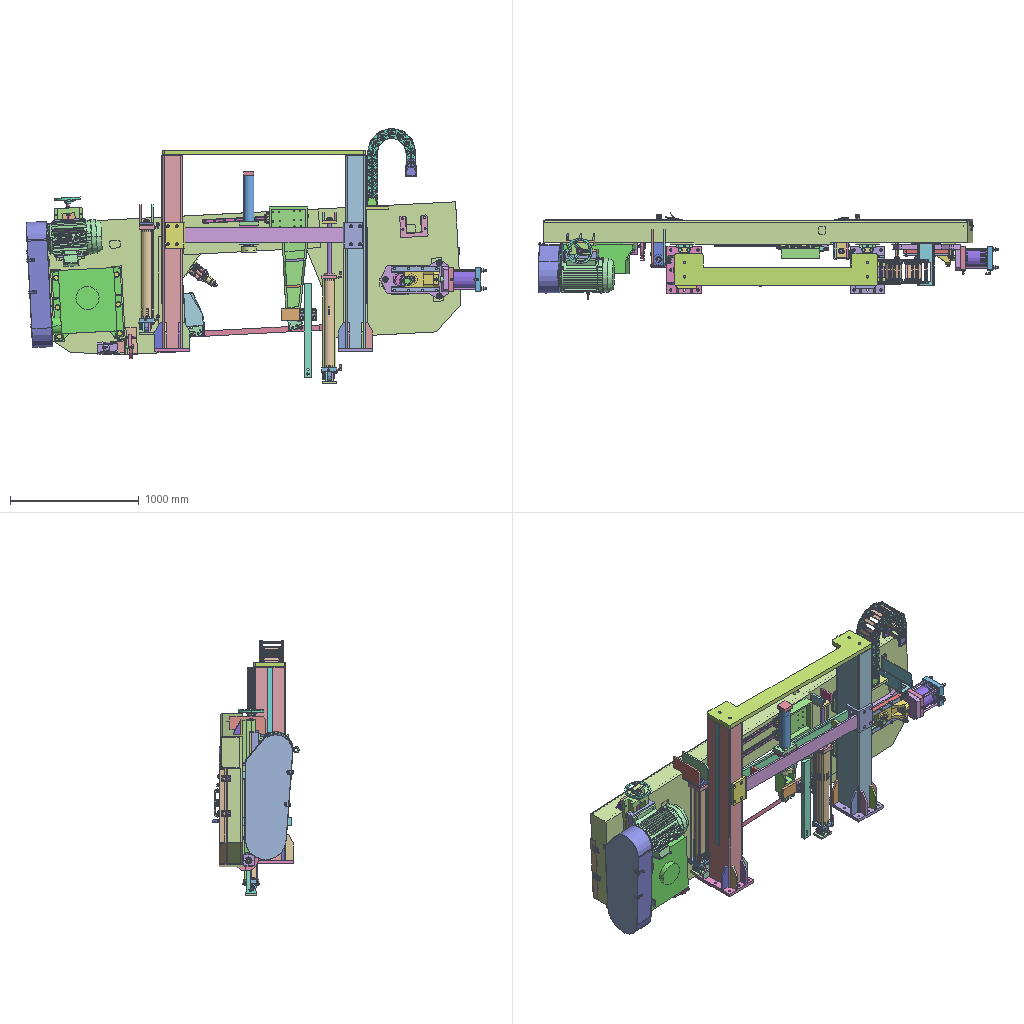Assembly | SolidWorks | 178 different items | 453 placed | box 3568 x 670 x 1981 mm
Parts list (item | name | quantity | parent item | size | volume | features):
1 | (subassembly) | x6 | in 21 | 75 x 44 x 44 mm | 50797 mm3 | -
2 | (subassembly) | x1 | - | - | 3103093 mm3 | features ReferencePattern 10, CompositeCurve 2, LocalChainPattern 1
3 | (subassembly) | x1 | in 2 | 145.118 x 185 x 82 mm | 205797 mm3 | features MirrorCompFeat 1, ReferencePattern 1
4 | (subassembly) | x11 | in 2 | 152 x 185 x 74 mm | 243841 mm3 | -
5 | (subassembly) | x1 | in 2 | 142.639 x 185 x 82 mm | 215082 mm3 | features MirrorCompFeat 1, ReferencePattern 1
6 | (subassembly) | x1 | - | 1530 x 622 x 137.5 mm | 11760878 mm3 | -
7 | (subassembly) | x1 | in 6 | 150 x 120 x 674.743 mm | 3033586 mm3 | -
8 | (subassembly) | x1 | - | - | 208271945 mm3 | features CompositeCurve 6
9 | (subassembly) | x1 | - | 159.892 x 293.5 x 1004 mm | 4407158 mm3 | features MirrorCompFeat 2, ReferencePattern 2
10 | (subassembly) | x1 | in 12 | 113.1 x 154 x 66 mm | 527835 mm3 | features ReferencePattern 4, MirrorCompFeat 1
11 | (subassembly) | x1 | in 9 | 159.892 x 127 x 873 mm | 2737891 mm3 | features ReferencePattern 9, LocalCirPattern 1
12 | (subassembly) | x1 | - | 1034 x 251 x 1320 mm | 13536578 mm3 | features CompositeCurve 1
13 | (subassembly) | x1 | - | 159.892 x 128.5 x 1129 mm | 3522058 mm3 | features MirrorCompFeat 2, ReferencePattern 2
14 | (subassembly) | x1 | in 12 | 113.1 x 154 x 66 mm | 527835 mm3 | features ReferencePattern 4, MirrorCompFeat 1
15 | (subassembly) | x1 | in 12 | 275 x 90 x 76.5 mm | 961874 mm3 | features ReferencePattern 13, LocalLPattern 1, MirrorCompFeat 1
16 | (subassembly) | x1 | - | 818.008 x 265.16 x 304.212 mm | 12071604 mm3 | features ReferencePattern 8, LocalLPattern 1, MirrorCompFeat 1
17 | (subassembly) | x6 | in 8 | 95.983 x 31.176 x 12 mm | 3413 mm3 | -
18 | (subassembly) | x1 | in 8 | 558.147 x 472.8 x 532.819 mm | 28170554 mm3 | features ReferencePattern 2, LocalLPattern 1, MirrorCompFeat 1
19 | (subassembly) | x1 | - | 1815 x 380 x 1565 mm | 40801474 mm3 | -
20 | (subassembly) | x1 | in 8 | 141.618 x 147.365 x 259.286 mm | 1445767 mm3 | -
21 | (subassembly) | x1 | in 8 | 690 x 549 x 426.5 mm | 59127815 mm3 | features ReferencePattern 3, MirrorCompFeat 1
22 | (subassembly) | x1 | in 13 | 159.892 x 127 x 1033 mm | 2737892 mm3 | features ReferencePattern 9, LocalCirPattern 1
23 | (subassembly) | x1 | in 8 | 280.7 x 140.048 x 94.951 mm | 1394120 mm3 | -
24 | (subassembly) | x1 | in 16 | 180 x 218.16 x 499.969 mm | 4201061 mm3 | features ReferencePattern 6, LocalCirPattern 1
25 | (subassembly) | x2 | in 8 | 90 x 42 x 820 mm | 939194 mm3 | features LocalLPattern 1, ReferencePattern 1
26 | (subassembly) | x1 | in 19 | 120 x 60 x 1330 mm | 3294670 mm3 | features LocalLPattern 1, ReferencePattern 1
27 | (subassembly) | x1 | in 19 | 120 x 60 x 1330 mm | 3294670 mm3 | features LocalLPattern 1, ReferencePattern 1
28 | (subassembly) | x8 | in 16 | 20 x 20 x 41.4 mm | 4793 mm3 | -
29 | (subassembly) | x4 | in 18 | 37.5 x 24 x 24 mm | 6610 mm3 | -
30 | (subassembly) | x4 | in 24 | 30 x 30 x 21.9 mm | 7598 mm3 | -
31 | - | x6 | in 17 | 56.004 x 15.265 x 22.5 mm | 1517 mm3 | features BaseBody 1
32 | - | x1 | in 24 | 180 x 180 x 56 mm | 1310949 mm3 | features ICE 4, RevCut 2, Extrusion 1, HoleWzd 1
33 | - | x1 | in 24 | 180 x 180 x 56 mm | 1375420 mm3 | features ICE 4, Extrusion 1, HoleWzd 1, RevCut 1
34 | - | x1 | in 24 | 40 x 150 x 150 mm | 516029 mm3 | features Chamfer 1, Revolution 1
35 | - | x1 | in 16 | 265 x 175 x 150 mm | 1974640 mm3 | features ICE 8, Chamfer 2, 3DProfileFeature 1, Extrusion 1, HoleWzd 1, RevCut 1
36 | - | x1 | in 16 | 526.008 x 205 x 304.212 mm | 5277088 mm3 | features ICE 7, HoleWzd 3, 3DProfileFeature 1, Extrusion 1, Fillet 1, WeldmentFeature 1
37 | - | x1 | in 18 | 45 x 200 x 200 mm | 211717 mm3 | features ICE 2, CirPattern 1, Revolution 1, Sweep 1
38 | - | x1 | - | 212 x 330 x 165 mm | 621985 mm3 | features ICE 3, Fillet 2, EdgeFlange 1, FlatPattern 1, HoleWzd 1, SMBaseFlange 1, SheetMetal 1
39 | - | x2 | in 8 | 138.654 x 37 x 27 mm | 43785 mm3 | features ICE 6, Extrusion 1
40 | - | x1 | in 8 | 34 x 10 x 100 mm | 16950 mm3 | features MBimport 1
41 | - | x1 | in 7 | 150 x 100 x 40 mm | 435431 mm3 | features ICE 3, Extrusion 1
42 | - | x2 | in 10, 14 | 6 x 6 x 26 mm | 614.212 mm3 | features Chamfer 2, Cut 2, Extrusion 1, RevCut 1, Revolution 1
43 | - | x1 | in 7 | 80 x 80 x 40 mm | 223172 mm3 | features Extrusion 1, ICE 1
44 | - | x1 | in 7 | 70 x 70 x 40 mm | 58905 mm3 | features Extrusion 1
45 | - | x1 | in 7 | 572 x 60 x 60 mm | 1573135 mm3 | features Revolution 1
46 | - | x1 | in 7 | 80 x 80 x 360 mm | 424115 mm3 | features Extrusion 1
47 | - | x1 | in 23 | 242.5 x 94.951 x 94.951 mm | 1199171 mm3 | features MBimport 1
48 | - | x1 | in 23 | 25 x 25 x 60 mm | 21851 mm3 | features Extrusion 1, ICE 1, RevCut 1
49 | - | x2 | in 18 | 50 x 290 x 20 mm | 282397 mm3 | features Extrusion 1, HoleWzd 1
50 | - | x1 | in 18 | 240 x 51 x 290 mm | 2244437 mm3 | features HoleWzd 2, Extrusion 1, ICE 1
51 | - | x1 | in 18 | 215 x 95 x 400 mm | 2889369 mm3 | features ICE 4, Extrusion 1, HoleWzd 1
52 | - | x1 | in 18 | 350.5 x 38 x 38 mm | 174413 mm3 | features Chamfer 1, ICE 1, Revolution 1
53 | - | x6 | in 10, 14 | 9 x 30 x 30 mm | 4367 mm3 | features Revolution 3, CirPattern 1, RefAxis 1
54 | - | x1 | in 18 | 50 x 60 x 73 mm | 158033 mm3 | features Chamfer 1, Extrusion 1, HoleWzd 1, ICE 1
55 | - | x2 | in 8 | 238 x 839.181 x 17 mm | 391508 mm3 | features Sweep 1
56 | - | x1 | in 8 | 163 x 973.632 x 386.5 mm | 1244808 mm3 | features ICE 7, Extrusion 1, HoleWzd 1, WeldBeadFeat 1, WeldmentFeature 1
57 | - | x2 | in 8 | 60 x 380 x 10 mm | 228000 mm3 | features Extrusion 1
58 | - | x1 | in 8 | 386.5 x 973.632 x 16 mm | 607839 mm3 | features ICE 3, Extrusion 1, WeldmentFeature 1
59 | - | x1 | - | 1570 x 250 x 35 mm | 9261323 mm3 | features SavedExtBody 1
60 | - | x1 | in 19 | 1570 x 250 x 35 mm | 9261323 mm3 | features Cut 2, Extrusion 1, Fillet 1
61 | - | x2 | in 10, 14 | 11 x 16 x 39 mm | 6238 mm3 | features ICE 2, Extrusion 1
62 | - | x2 | in 9, 13 | 47 x 22 x 47 mm | 19543 mm3 | features Revolution 2
63 | - | x3 | in 16 | 128 x 36 x 41.569 mm | 67364 mm3 | features ICE 2, Extrusion 1, RevCut 1, Revolution 1
64 | - | x8 | in 15 | 11 x 35 x 35 mm | 6620 mm3 | features Revolution 3, CirPattern 1, RefAxis 1
65 | - | x1 | in 8 | 75 x 110 x 110 mm | 369149 mm3 | features HoleWzd 1, ICE 1, Revolution 1
66 | - | x1 | in 23 | 205 x 30 x 190 mm | 425990 mm3 | features ICE 1, MBimport 1
67 | - | x1 | in 23 | 90 x 140.048 x 92.376 mm | 160839 mm3 | features ICE 4, BossThin 1, Extrusion 1
68 | - | x1 | in 24 | 160 x 160 x 170 mm | 413905 mm3 | features Extrusion 1
69 | - | x1 | in 24 | 310 x 40 x 40 mm | 342944 mm3 | features Chamfer 1, Fillet 1, ICE 1, Revolution 1
70 | - | x1 | in 8 | 3295 x 1050 x 195 mm | 87655844 mm3 | features ICE 22, HoleWzd 5, BossThin 4, Cut 3, Rib 2, Extrusion 1, Fillet 1, WeldmentFeature 1
71 | - | x1 | - | 84.105 x 48.48 x 5.05 mm | 14009 mm3 | features SplitBody 1
72 | - | x1 | - | 45 x 38 x 1330 mm | 1945427 mm3 | features SplitBody 1
73 | - | x1 | in 19 | 395 x 1530 x 370 mm | 12639229 mm3 | features ICE 8, HoleWzd 4, Cut 2, MirrorSolid 2, Fillet 1, WeldMemberFeat 1, WeldmentFeature 1
74 | - | x1 | in 19 | 270 x 1530 x 370 mm | 12311582 mm3 | features ICE 8, HoleWzd 3, MirrorSolid 2, WeldMemberFeat 1, WeldmentFeature 1
75 | - | x2 | in 18 | 47 x 15 x 47 mm | 13242 mm3 | features Revolution 3, CirPattern 1, Fillet 1
76 | - | x8 | in 11, 22 | 760.5 x 20.785 x 18 mm | 86944 mm3 | features RevCut 3, CirPattern 1, Cut 1, Extrusion 1, Fillet 1, LPattern 1, Revolution 1
77 | - | x1 | in 23 | 37.3 x 32.303 x 20.2 mm | 12259 mm3 | features Cut 2, Chamfer 1, Extrusion 1
78 | - | x1 | in 24 | 40 x 17.321 x 15 mm | 4755 mm3 | features ICE 2, Boss 1, RevCut 1, Revolution 1
79 | - | x4 | in 11, 22 | 18 x 38.892 x 47.244 mm | 8990 mm3 | features Boss 4, Fillet 2, RevCut 2, Revolution 2, Chamfer 1, ICE 1, Sweep 1
80 | - | x1 | in 24 | 42.66 x 42.66 x 15 mm | 7800 mm3 | features Boss 5, RevCut 5, Fillet 2, ICE 2, Revolution 2, Sweep 1
81 | - | x2 | in 11, 22 | 115 x 115 x 60 mm | 477464 mm3 | features ICE 4, Extrusion 1, HoleWzd 1, RevCut 1
82 | - | x8 | in 28 | 41.4 x 18.475 x 16 mm | 4096 mm3 | features Chamfer 2, RevCut 2, Revolution 2, Extrusion 1, ICE 1
83 | - | x6 | in 1 | 75 x 41.569 x 36 mm | 43357 mm3 | features Chamfer 2, RevCut 2, Revolution 2, Extrusion 1, ICE 1
84 | - | x4 | in 29 | 37.5 x 20.785 x 18 mm | 5393 mm3 | features Chamfer 2, RevCut 2, Revolution 2, Extrusion 1, ICE 1
85 | - | x4 | in 30 | 24 x 27.713 x 14.8 mm | 5128 mm3 | features Cut 2, Extrusion 1
86 | - | x4 | in 16 | 155 x 24 x 24 mm | 33595 mm3 | features BlendCut 1, Chamfer 1, Cut 1, Fillet 1, ICE 1, LPattern 1, RevCut 1, Revolution 1
87 | - | x4 | in 10, 14 | 16 x 10 x 10 mm | 686.381 mm3 | features BlendCut 1, Cut 1, Fillet 1, LPattern 1, RevCut 1, Revolution 1
88 | - | x4 | in 10, 14 | 28 x 13 x 13 mm | 1937 mm3 | features BlendCut 1, Cut 1, Fillet 1, LPattern 1, RevCut 1, Revolution 1
89 | - | x2 | in 10, 14 | 10 x 8 x 8 mm | 407.497 mm3 | features RevCut 2, Cut 1, LPattern 1, Revolution 1
90 | - | x16 | in 10, 14 | 20 x 8 x 8 mm | 910.152 mm3 | features RevCut 2, Cut 1, LPattern 1, Revolution 1
91 | - | x8 | in 9, 13 | 44.721 x 44.721 x 10 mm | 9603 mm3 | features Chamfer 3, CirPattern 1, Cut 1, Extrusion 1
92 | - | x2 | in 11, 22 | 115 x 115 x 118 mm | 524654 mm3 | features ICE 6, HoleWzd 4, Extrusion 1, RevCut 1
93 | - | x2 | in 8 | 71.554 x 71.554 x 12 mm | 25041 mm3 | features Chamfer 3, CirPattern 1, Cut 1, Extrusion 1
94 | - | x1 | in 6 | 77.589 x 77.589 x 12 mm | 27297 mm3 | features Chamfer 3, CirPattern 1, Cut 1, Extrusion 1
95 | - | x2 | in 8 | 94.663 x 94.663 x 12 mm | 44617 mm3 | features Chamfer 3, CirPattern 1, Cut 1, Extrusion 1
96 | - | x2 | in 21 | 104.523 x 104.523 x 15 mm | 66046 mm3 | features Chamfer 3, CirPattern 1, Cut 1, Extrusion 1
97 | - | x8 | in 28 | 16.182 x 16.166 x 2 mm | 241.9 mm3 | features Extrusion 1
98 | - | x4 | in 10, 14 | 11.5 x 13.997 x 1 mm | 53.264 mm3 | features Extrusion 1
99 | - | x4 | in 29 | 18.367 x 18.334 x 3.1 mm | 444.091 mm3 | features Extrusion 1
100 | - | x4 | in 30 | 24.356 x 24.313 x 4.1 mm | 1031 mm3 | features Extrusion 1
101 | - | x8 | in 11, 22 | 30.149 x 30.097 x 5 mm | 1905 mm3 | features Extrusion 1
102 | - | x6 | in 1 | 36.439 x 36.377 x 6 mm | 3321 mm3 | features Extrusion 1
103 | - | x2 | in 11, 22 | 755 x 32 x 32 mm | 580870 mm3 | features Revolution 1
104 | - | x4 | in 29 | 24 x 2.5 x 24 mm | 773.126 mm3 | features Revolution 1
105 | - | x8 | in 11, 22 | 37 x 3 x 37 mm | 2085 mm3 | features Revolution 1
106 | - | x4 | in 24 | 304 x 16 x 16 mm | 49717 mm3 | features MirrorPattern 2, LPattern 1, RevCut 1, Revolution 1
107 | - | x8 | in 28 | 20 x 20 x 2 mm | 455.138 mm3 | features Extrusion 1
108 | - | x4 | in 30 | 30 x 30 x 3 mm | 1440 mm3 | features Extrusion 1
109 | - | x6 | in 1 | 44 x 44 x 4 mm | 4119 mm3 | features Extrusion 1
110 | - | x4 | in 25 | 90 x 36.5 x 125.4 mm | 221238 mm3 | features ICE 22, Extrusion 5, MirrorPattern 5, Fillet 4, MirrorSolid 4, Chamfer 3, RevCut 3, Dome 2, LPattern 2, Revolution 2, DeleteBody 1, LibraryFeature 1
111 | - | x2 | in 25 | 28 x 26 x 820 mm | 496717 mm3 | features ICE 19, MirrorPattern 5, Extrusion 4, MirrorSolid 4, Chamfer 3, Fillet 3, RevCut 3, Dome 2, LPattern 2, DeleteBody 1, LibraryFeature 1, Revolution 1
112 | - | x4 | in 26, 27 | 120 x 50.5 x 197.1 mm | 674621 mm3 | features ICE 22, Extrusion 5, MirrorPattern 5, Fillet 4, MirrorSolid 4, Chamfer 3, RevCut 3, Dome 2, LPattern 2, Revolution 2, CreateAssemFeat 1, DeleteBody 1, LibraryFeature 1
113 | - | x2 | in 26, 27 | 45 x 38 x 1330 mm | 1945427 mm3 | features ICE 19, MirrorPattern 5, Extrusion 4, MirrorSolid 4, Chamfer 3, Fillet 3, RevCut 3, Dome 2, LPattern 2, CreateAssemFeat 1, DeleteBody 1, LibraryFeature 1, Revolution 1
114 | - | x2 | in 11, 22 | 60 x 90 x 90 mm | 271909 mm3 | features Chamfer 1, Revolution 1
115 | - | x22 | in 4 | 152 x 31.5 x 74 mm | 87021 mm3 | features BaseBody 1
116 | - | x2 | in 3 | 145.118 x 31.5 x 82 mm | 67988 mm3 | features ICE 3, BaseBody 1
117 | - | x2 | in 5 | 142.639 x 31.5 x 82 mm | 72646 mm3 | features ICE 3, BaseBody 1
118 | - | x26 | in 3, 4, 5 | 150 x 9.3 x 38 mm | 34912 mm3 | features Extrusion 1, Fillet 1, ICE 1, MirrorPattern 1
119 | - | x1 | in 2 | - | - | -
120 | - | x1 | in 18 | 505 x 319.8 x 355 mm | 20440913 mm3 | features ICE 21, CirPattern 7, LibraryFeature 7, Extrusion 6, Fillet 6, RevCut 6, Revolution 5, Chamfer 4, CombineBodies 3, MoveCopyBody 3, CurvePattern 2, DeleteBody 2, MirrorSolid 2, CutThin 1, RevCutThin 1
121 | - | x4 | in 8 | 69 x 50 x 13 mm | 23385 mm3 | features BaseBody 3
122 | - | x1 | in 6 | 1530 x 200 x 135 mm | 8097209 mm3 | features ICE 6, Fillet 2, Extrusion 1, HoleWzd 1, MirrorSolid 1, WeldmentFeature 1
123 | - | x1 | in 6 | 25 x 115 x 150 mm | 301393 mm3 | features Extrusion 1, HoleWzd 1, ICE 1
124 | - | x1 | in 6 | 25 x 115 x 150 mm | 301393 mm3 | features Extrusion 1, HoleWzd 1, ICE 1
125 | - | x2 | in 11, 22 | 95 x 95 x 690 mm | 501280 mm3 | features Extrusion 1
126 | - | x1 | in 7 | 120 x 120 x 40 mm | 318828 mm3 | features ICE 3, CirPattern 1, Extrusion 1
127 | - | x1 | in 18 | 135 x 170 x 170 mm | 1424823 mm3 | features HoleWzd 1, ICE 1, Revolution 1
128 | - | x1 | in 18 | 45 x 45 x 6 mm | 9126 mm3 | features Chamfer 1, Extrusion 1
129 | - | x1 | in 8 | 75 x 660 x 660 mm | 8495500 mm3 | features Fillet 2, HoleWzd 2, Blend 1, CirPattern 1, ICE 1, Revolution 1
130 | - | x1 | in 21 | 135 x 240 x 240 mm | 3122246 mm3 | features HoleWzd 1, ICE 1, Revolution 1
131 | - | x1 | in 21 | 45 x 45 x 6 mm | 8937 mm3 | features Chamfer 1, Extrusion 1
132 | - | x1 | in 8 | 74 x 74 x 260 mm | 722513 mm3 | features Chamfer 1, Extrusion 1, RevCut 1
133 | - | x1 | in 8 | 75 x 660 x 660 mm | 8244965 mm3 | features CirPattern 2, Fillet 2, HoleWzd 2, Blend 1, ICE 1, Revolution 1
134 | - | x1 | in 8 | 36 x 170 x 170 mm | 217484 mm3 | features Chamfer 1, HoleWzd 1, Revolution 1
135 | - | x1 | in 12 | 300 x 880.131 x 235 mm | 7902209 mm3 | features ICE 9, Chamfer 1, Cut 1, Extrusion 1, Shell 1, WeldmentFeature 1
136 | - | x6 | in 17 | 58.8 x 15.3 x 12 mm | 930.521 mm3 | features BaseBody 1
137 | - | x1 | - | 300 x 880.131 x 235 mm | 7902209 mm3 | features ICE 9, Chamfer 1, Cut 1, Extrusion 1, Shell 1, WeldmentFeature 1
138 | - | x1 | - | 84.105 x 48.48 x 15 mm | 44236 mm3 | features SplitBody 1
139 | - | x1 | - | 120 x 50.5 x 128.8 mm | 512152 mm3 | features SplitBody 1
140 | - | x1 | - | 84.105 x 48.965 x 15.15 mm | 44523 mm3 | features SplitBody 1
141 | - | x1 | - | 84.105 x 48.965 x 15.15 mm | 44523 mm3 | features SplitBody 1
142 | - | x1 | - | - | - | -
143 | - | x1 | - | 84.105 x 48.48 x 5.05 mm | 14009 mm3 | features SplitBody 1
144 | - | x1 | - | 15 x 30 x 10 mm | 2949 mm3 | features Extrusion 1
145 | - | x1 | in 9 | 110 x 280 x 156 mm | 1285490 mm3 | features ICE 3, Chamfer 1, Extrusion 1, MirrorSolid 1, WeldmentFeature 1
146 | - | x1 | in 13 | 110 x 115 x 81 mm | 400390 mm3 | features ICE 3, Extrusion 1, MirrorSolid 1, WeldmentFeature 1
147 | - | x6 | in 17 | 31.176 x 19.62 x 8.2 mm | 515.875 mm3 | features BaseBody 1
148 | - | x2 | in 9, 13 | 110 x 90 x 86.592 mm | 265530 mm3 | features ICE 2, Extrusion 1, MirrorSolid 1
149 | - | x2 | in 9, 13 | 88 x 33 x 33 mm | 60292 mm3 | features Chamfer 1, Revolution 1
150 | - | x1 | in 8 | 980 x 794 x 53 mm | 2935237 mm3 | features HoleWzd 2, ICE 2, BossThin 1, Cut 1, ExtruThin 1
151 | - | x1 | in 12 | 140 x 255 x 130 mm | 2115971 mm3 | features ICE 4, HoleWzd 2, Extrusion 1
152 | - | x1 | in 12 | 140 x 257 x 134 mm | 207970 mm3 | features ICE 2, ExtruThin 1, WeldmentFeature 1
153 | - | x1 | - | 17.303 x 10 x 16.688 mm | 1169 mm3 | features SplitBody 1
154 | - | x2 | in 8 | 24.75 x 120 x 120 mm | 131163 mm3 | features BaseBody 1
155 | - | x4 | in 10, 14 | 66 x 10 x 35 mm | 21292 mm3 | features Fillet 3, Extrusion 1, HoleWzd 1, ICE 1
156 | - | x2 | in 10, 14 | 60 x 18 x 18 mm | 5416 mm3 | features ICE 6, Chamfer 1, Extrusion 1
157 | - | x2 | in 10, 14 | 78 x 18 x 18 mm | 8414 mm3 | features ICE 6, Chamfer 1, Extrusion 1
158 | - | x6 | in 17 | 29.742 x 26.5 x 2.5 mm | 449.782 mm3 | features BaseBody 1
159 | - | x2 | in 10, 14 | 102 x 152 x 66 mm | 438428 mm3 | features ICE 6, HoleWzd 5, Chamfer 1, Extrusion 1, MirrorPattern 1
160 | - | x4 | in 15 | 22 x 22 x 53 mm | 9954 mm3 | features Chamfer 1, Extrusion 1, ICE 1
161 | - | x1 | in 8 | 1000 x 744 x 53 mm | 2674985 mm3 | features HoleWzd 2, Cut 1, ExtruThin 1, ICE 1
162 | - | x1 | in 15 | 136 x 90 x 25 mm | 286183 mm3 | features Extrusion 1, ICE 1
163 | - | x1 | in 12 | 30 x 60 x 725 mm | 1292936 mm3 | features Cut 1, Extrusion 1, ICE 1
164 | - | x1 | in 15 | 275 x 90 x 23.5 mm | 580616 mm3 | features Extrusion 1
165 | - | x4 | in 15 | 22 x 22 x 3 mm | 574.322 mm3 | features Extrusion 1
166 | - | x1 | in 8 | 3091 x 670.5 x 43 mm | 356938 mm3 | features Blend 2, ICE 1, Sweep 1
167 | - | x2 | in 16 | 370 x 34 x 10 mm | 121999 mm3 | features Extrusion 1
168 | - | x1 | in 8 | 75 x 109 x 215 mm | 446232 mm3 | features Extrusion 1, HoleWzd 1, ICE 1, LPattern 1, WeldmentFeature 1
169 | - | x1 | in 21 | 635 x 540 x 409 mm | 55559758 mm3 | features ICE 15, Extrusion 1, LPattern 1, MirrorPattern 1
170 | Cage.STEP | x1 | - | - | - | -
171 | Component2.STEP | x1 | - | - | - | -
172 | Component3-0.STEP | x1 | - | - | - | -
173 | Component3.STEP (subassembly) | x1 | - | - | - | -
174 | Component4.STEP | x1 | - | - | - | -
175 | Fox X2 222.3 v56.STEP | x1 | - | - | - | -
176 | - | x1 | - | - | - | -
177 | damper fox x2 float.STEP (subassembly) | x1 | - | - | - | -
178 | 红外线感应.STEP (subassembly) | x1 | - | - | - | -
Mates (type | each side: item.copy, entity, surface, feature), first 465 of 527 lines:
In the top assembly
Coincident | 145.1 face plane Boss-Extrude 3 | 70.1 face plane Boss-Extrude 1
Coincident | 146.1 face plane Boss-Extrude 3 | 70.1 face plane Boss-Extrude 1
Coincident | 145.1 edge | 70.1 face plane Boss-Extrude 1
DistanceDim | 146.1 vertex | 70.1 face plane Boss-Extrude 1
Coincident | 70.1 face plane Boss-Extrude 1 | 38.1 face plane Boss-Extrude 1
Coincident | 70.1 face plane Cut-Extrude 11 | 38.1 face plane Base-Flange 1
Coincident | 73.1 face plane Rhs RHS250X150X6.3(1) | 122.1 face plane Mirror 1 | 2 times
Concentric | 73.1 face cylinder Cut-Extrude 1 | 122.1 face cylinder Mirror 1 | 2 times
DistanceDim | 148.1 face plane Boss-Extrude 1 | 73.1 face plane Boss-Extrude 1
Concentric | 73.1 face cylinder M8x1.0 Tapped Hole 1 | 116.1 face cylinder Boss-Extrude 3
Concentric | 73.1 face cylinder M8x1.0 Tapped Hole 1 | 116.2 face cylinder Boss-Extrude 3
Coincident | 73.1 face plane Boss-Extrude 6 | 116.1 face plane 输入1
DistanceDim | 148.2 face plane Boss-Extrude 1 | 74.1 face plane Boss-Extrude 1
Coincident | 70.1 face plane Boss-Extrude 10 | 112.1 face plane Boss-Extrude 1
Concentric | 70.1 face cylinder M14 Tapped Hole 3 | 112.1 face cylinder Mirror 2
Concentric | 70.1 face cylinder M14 Tapped Hole 3 | 112.2 face cylinder Mirror 1
Parallel | 166.1 face plane Boss-Extrude 1 | 135.1 face plane Boss-Extrude 2
Coincident | 70.1 face plane Boss-Extrude 1 | 135.1 face plane Boss-Extrude 2
Coincident | 70.1 face plane Boss-Extrude 12 | 36.1 face plane Boss-Extrude 1
Concentric | 70.1 edge | 36.1 face cylinder Boss-Extrude 7
In subassembly 9
Concentric | 148.3 face cylinder Cut-Extrude 1 | 92.1 face cylinder Boss-Extrude 3
Concentric | 149.1 face cylinder Revolve 1 | 148.3 face cylinder Mirror 1
Width | 148.3 face plane Mirror 1 | 148.3 face plane Boss-Extrude 2 | 92.1 face plane Boss-Extrude 3 | 92.1 face plane Boss-Extrude 3
Coincident | 149.1 face plane Revolve 1 | 148.3 face plane Boss-Extrude 2
Concentric | 145.2 face cylinder Cut-Extrude 1 | 103.1 face cylinder Revolve 1
Coincident | 145.2 face plane Boss-Extrude 1 | 103.1 face plane Revolve 1
Concentric | 103.1 face cylinder Revolve 1 | 91.1 face cylinder Base-Extrude
Coincident | 145.2 face plane Boss-Extrude 1 | 91.1 face plane Base-Extrude
Concentric | 149.1 face cylinder Revolve 1 | 91.2 face cylinder Base-Extrude
Coincident | 148.3 face plane Mirror 1 | 91.2 face plane Base-Extrude
Concentric | 92.1 face cylinder Boss-Extrude 3 | 62.1 face cylinder Revolve 2
Width | 92.1 face plane Boss-Extrude 3 | 92.1 face plane Boss-Extrude 3 | 62.1 face plane Revolve 1 | 62.1 face plane Revolve 1
Coincident | 11.1 plane | 9.1 plane | 3 times
Parallel | 145.2 face plane Boss-Extrude 3 | 81.1 face plane Boss-Extrude 1
In subassembly 11
Coincident | 92.2 plane | 11.2 plane | 3 times
Concentric | 125.1 face cylinder Boss-Extrude 1 | 92.2 face cylinder Boss-Extrude 2
Coincident | 125.1 face plane Boss-Extrude 1 | 92.2 face plane Boss-Extrude 1
Concentric | 103.2 face cylinder Revolve 1 | 114.1 face cylinder Revolve 1
DistanceDim | 103.2 face plane Revolve 1 | 114.1 face plane Revolve 1
Concentric | 125.1 face cylinder Boss-Extrude 1 | 114.1 face cylinder Revolve 1
Concentric | 125.1 face cylinder Boss-Extrude 1 | 81.2 face cylinder Boss-Extrude 2
Coincident | 125.1 face plane Boss-Extrude 1 | 81.2 face plane Boss-Extrude 1
LimitDistanceDim | 92.2 face plane Boss-Extrude 2 | 114.1 face plane Revolve 1
Concentric | 92.2 face cylinder Boss-Extrude 1 | 76.1 face cylinder Boss-Revolve 1
Concentric | 76.1 face cylinder Boss-Revolve 1 | 105.1 face cylinder Base-Revolve
Concentric | 76.1 face cylinder Boss-Revolve 1 | 101.1 face cylinder Extrude 1
Coincident | 92.2 face plane Boss-Extrude 1 | 105.1 face plane Base-Revolve
Coincident | 105.1 face plane Base-Revolve | 101.1 face plane Extrude 1
Coincident | 76.1 face plane Base-Extrude | 101.1 face plane Extrude 1
Concentric | 92.2 face cone 1/4 Rc Tapped Hole 1 | 79.1 face cone Revolve 2
Coincident | 92.2 face plane Boss-Extrude 1 | 79.1 face plane Revolve 2
Concentric | 81.2 face cylinder Boss-Extrude 1 | 76.1 face cylinder Boss-Revolve 1
Concentric | 81.2 face cone 1/4 NPT Tapped Hole 2 | 79.2 face cone Revolve 2
Coincident | 81.2 face plane Boss-Extrude 1 | 79.2 face plane Revolve 2
In subassembly 8
Coincident | 70.2 face plane Boss-Extrude 8 | 161.1 face plane Extrude-薄壁1
Concentric | 70.2 face cylinder Boss-Extrude 1 | 169.1 face cylinder Boss-Extrude 9
Coincident | 70.2 plane | 8.1 plane | 3 times
Coincident | 70.2 face plane Boss-Extrude 11 | 169.1 face plane Boss-Extrude 1
Parallel | 70.2 face plane Boss-Extrude 11 | 169.1 face plane Boss-Extrude 1
Coincident | 70.2 face plane Boss-Extrude 1 | 51.1 face plane Boss-Extrude 1
Concentric | 129.1 face cylinder Revolve 1 | 169.1 face cylinder Boss-Extrude 12
Concentric | 129.1 face cylinder Revolve 1 | 65.1 face cylinder Revolve 1
Concentric | 129.1 face cylinder M10 Tapped Hole 2 | 65.1 face cylinder M10 Tapped Hole 1
Coincident | 129.1 face plane Revolve 1 | 65.1 face plane Revolve 1
Coincident | 70.2 face plane Boss-Extrude 12 | 8.1 face
Concentric | 133.1 face cylinder M6 Tapped Hole 1 | 134.1 face cylinder M6 间隙Hole 1
Coincident | 133.1 face plane Revolve 1 | 134.1 face plane Revolve 1
Concentric | 133.1 face cylinder Revolve 1 | 134.1 face cylinder Revolve 1
Coincident | 70.2 face plane Boss-Extrude 1 | 8.1 face | 2 times
Tangent | 70.2 face plane Boss-Extrude 12 | 8.1 face
Concentric | 70.2 face cylinder Cut-Extrude 13 | 8.1 face
Concentric | 8.1 face | 8.1 face | 2 times
Parallel | 8.1 face | 8.1 face | 2 times
Concentric | 70.2 face cylinder Cut-Extrude 15 | 111.1 face cylinder LPattern 1
Concentric | 70.2 face cylinder Cut-Extrude 15 | 111.2 face cylinder LPattern 1
Coincident | 110.1 face plane Mirror 17 | 110.2 face plane Mirror 17
Concentric | 70.2 face cylinder Cut-Extrude 15 | 111.2 face cylinder Cut-Revolve 2
Concentric | 70.2 face cylinder Cut-Extrude 15 | 111.1 face cylinder Cut-Revolve 2
Width | 8.1 face | 8.1 face | 70.2 face plane Boss-Extrude 14 | 70.2 face plane Boss-Extrude 1
Coincident | 70.2 face plane Boss-Extrude 1 | 168.1 face plane Boss-Extrude 1
Coincident | 51.1 face plane Boss-Extrude 1 | 168.1 face plane Boss-Extrude 1 | 2 times
Coincident | 8.1 face | 8.1 face | 4 times
Concentric | 133.1 face cylinder Revolve 1 | 166.2 face cylinder Sweep 2
Coincident | 133.1 face plane Revolve 1 | 166.2 face plane Sweep 2
Coincident | 130.1 face plane Revolve 1 | 127.1 face plane Revolve 1
Concentric | 130.1 face cylinder Revolve 1 | 56.1 face cylinder Boss-Extrude 2
Parallel | 70.2 face plane Boss-Extrude 1 | 56.1 face plane Boss-Extrude 2
DistanceDim | 129.1 face plane Revolve 1 | 70.2 face plane Boss-Extrude 1
Concentric | 8.1 face | 132.1 face cylinder Cut-Revolve 1
Coincident | 8.1 face | 132.1 face plane Cut-Revolve 1
Coincident | 133.1 face plane Revolve 1 | 129.1 face plane Revolve 1
Coincident | 8.1 face | 40.1 face plane 水枪.STEP<1>
Concentric | 8.1 face | 40.1 face cylinder 水枪.STEP<1>
Concentric | 127.1 face cylinder Revolve 1 | 55.1 select_type:24
Coincident | 127.1 face cone Revolve 1 | 55.1 edge
Concentric | 130.1 edge | 55.1 face cylinder Sweep 1
Slot | 70.2 face cylinder Boss-Extrude 1 | 132.1 face cylinder Cut-Revolve 1
Concentric | 133.1 face cylinder Revolve 1 | 132.1 face cylinder Cut-Revolve 1
Concentric | 127.1 face cylinder Revolve 1 | 55.2 face cylinder Sweep 1
Concentric | 130.1 face cylinder Revolve 1 | 55.2 face cylinder Sweep 1
Coincident | 130.1 face cone Revolve 1 | 55.2 edge
Coincident | 56.1 face plane Boss-Extrude 3 | 57.1 face plane Boss-Extrude 1
Coincident | 70.2 face plane Boss-Extrude 1 | 57.1 face plane Boss-Extrude 1
DistanceDim | 57.1 face plane Boss-Extrude 1 | 70.2 face plane Boss-Extrude 11
Coincident | 56.1 face plane Boss-Extrude 3 | 57.2 face plane Boss-Extrude 1
Coincident | 70.2 face plane Boss-Extrude 1 | 57.2 face plane Boss-Extrude 1
DistanceDim | 57.2 face plane Boss-Extrude 1 | 57.1 face plane Boss-Extrude 1
DistanceDim | 57.2 face plane Boss-Extrude 1 | 70.2 face plane Boss-Extrude 1
Coincident | 161.1 face plane Boss-Extrude 1 | 39.1 face plane Boss-Extrude 1
DistanceDim | 39.1 face plane Boss-Extrude 1 | 161.1 face plane Extrude-薄壁1
Coincident | 150.1 face plane Extrude-薄壁1 | 39.2 face plane Boss-Extrude 1
DistanceDim | 39.2 face cylinder Boss-Extrude 2 | 70.2 face plane Boss-Extrude 3
DistanceDim | 39.1 face cylinder Boss-Extrude 2 | 70.2 face plane Boss-Extrude 3
Concentric | 132.1 face cylinder Cut-Revolve 1 | 154.1 face cylinder 输入1
Coincident | 132.1 face plane Cut-Revolve 1 | 154.1 face plane 输入1
Concentric | 132.1 face cylinder Cut-Revolve 1 | 154.2 face cylinder 输入1
Coincident | 133.1 face plane Revolve 1 | 154.2 face plane 输入1
Concentric | 132.1 face cylinder Cut-Revolve 1 | 93.1 face cylinder Base-Extrude
Concentric | 132.1 face cylinder Cut-Revolve 1 | 93.2 face cylinder Base-Extrude
Coincident | 93.1 face plane Base-Extrude | 93.2 face plane Base-Extrude
Concentric | 132.1 face cylinder Cut-Revolve 1 | 95.1 face cylinder Base-Extrude
Coincident | 95.1 face plane Base-Extrude | 95.2 face plane Base-Extrude
Concentric | 95.1 face cylinder Base-Extrude | 95.2 face cylinder Base-Extrude
Coincident | 154.2 face plane 输入1 | 95.2 face plane Base-Extrude
Coincident | 56.1 face plane Cut-Extrude 1 | 58.1 face plane Boss-Extrude 1
Concentric | 56.1 face cylinder Boss-Extrude 2 | 58.1 face cylinder Boss-Extrude 1
Coincident | 161.1 face plane Extrude-薄壁1 | 121.1 face plane 输入3
Coincident | 70.2 face plane Boss-Extrude 1 | 121.1 face plane 输入2
DistanceDim | 121.1 face plane 输入3 | 161.1 face plane Boss-Extrude 1
DistanceDim | 121.1 face plane 输入3 | 161.1 face plane Extrude-薄壁1
Coincident | 70.2 face plane Boss-Extrude 1 | 121.2 face plane 输入2
DistanceDim | 121.2 face plane 输入2 | 121.1 edge
Coincident | 121.1 face plane 输入3 | 121.2 face plane 输入3
Coincident | 70.2 face plane Boss-Extrude 1 | 121.3 face plane 输入3
Coincident | 70.2 face plane Boss-Extrude 1 | 121.4 face plane 输入2
Coincident | 121.3 face plane 输入2 | 121.4 face plane 输入2
DistanceDim | 121.3 face plane 输入3 | 121.4 face plane 输入3
Coincident | 70.2 face plane Boss-Extrude 1 | 47.1 face plane 电机90W4级.STEP<1>
DistanceDim | 47.1 face plane 电机90W4级.STEP<1> | 70.2 face plane Boss-Extrude 1
Coincident | 70.2 face plane Boss-Extrude 1 | 161.1 face plane Extrude-薄壁1
Coincident | 8.1 face | 93.1 face plane Base-Extrude
Slot | 133.1 face cylinder Revolve 1 | 70.2 face cylinder Boss-Extrude 1
Coincident | 70.2 face plane Boss-Extrude 9 | 150.1 face plane Extrude-薄壁1
Coincident | 70.2 face plane Boss-Extrude 1 | 150.1 face plane Extrude-薄壁1
DistanceDim | 121.3 face plane 输入2 | 150.1 face plane Extrude-薄壁1 | 2 times
Coincident | 56.1 face plane Boss-Extrude 2 | 136.1 face plane 输入1
Coincident | 58.1 face plane Boss-Extrude 1 | 147.1 face plane 输入1
Coincident | 56.1 face plane Boss-Extrude 6 | 58.1 face plane Boss-Extrude 3
Coincident | 56.1 face plane Boss-Extrude 2 | 136.2 face plane 输入1
Coincident | 58.1 face plane Boss-Extrude 1 | 147.2 face plane 输入1
DistanceDim | 39.2 face plane Boss-Extrude 1 | 150.1 face plane Extrude-薄壁1
Coincident | 150.1 face plane Extrude-薄壁1 | 136.3 face plane 输入1
Width | 31.1 face plane 输入1 | 31.1 face plane 输入1 | 70.2 face plane Boss-Extrude 13 | 70.2 face plane Boss-Extrude 13
Coincident | 150.1 face plane Extrude-薄壁1 | 121.3 face plane 输入2
Coincident | 70.2 face plane Boss-Extrude 13 | 147.3 face plane 输入1
DistanceDim | 70.2 face plane Cut-Extrude 16 | 47.1 face plane 电机90W4级.STEP<1>
Coincident | 161.1 face plane Boss-Extrude 1 | 136.4 face plane 输入1
Coincident | 161.1 face plane Boss-Extrude 1 | 136.5 face plane 输入1
Coincident | 70.2 face plane Boss-Extrude 15 | 147.4 face plane 输入1
Coincident | 70.2 face plane Boss-Extrude 15 | 147.5 face plane 输入1
Coincident | 150.1 face plane Extrude-薄壁1 | 136.6 face plane 输入1
Coincident | 70.2 face plane Boss-Extrude 13 | 147.6 face plane 输入1
Concentric | 70.2 face cylinder Cut-Extrude 17 | 147.6 face cylinder 输入1
Concentric | 70.2 face cylinder Cut-Extrude 17 | 147.3 face cylinder 输入1
Concentric | 56.1 face cylinder M5 Tapped Hole 1 | 136.1 face cylinder 输入1 | 2 times
Concentric | 56.1 face cylinder M5 Tapped Hole 1 | 136.2 face cylinder 输入1 | 2 times
Concentric | 70.2 face cylinder Cut-Extrude 19 | 147.4 face cylinder 输入1 | 2 times
Concentric | 70.2 face cylinder Cut-Extrude 19 | 147.5 face cylinder 输入1 | 2 times
DistanceDim | 70.2 face plane Extrude-薄壁1 | 8.1 edge
Coincident | 70.2 face plane Cut-Extrude 20 | 111.1 face plane Boss-Extrude 10
Coincident | 70.2 face plane Cut-Extrude 20 | 111.2 face plane Boss-Extrude 10
PlanarAngleDim | 70.2 face plane Boss-Extrude 1 | 8.1 face
Coincident | 8.1 face | 110.1 face plane Boss-Extrude 1
Coincident | 8.1 vertex | 110.1 face plane Mirror 17
DistanceDim | 70.2 face plane Boss-Extrude 1 | 8.1 edge
In subassembly 25
Coincident | 110.3 face plane Cut-Extrude 11 | 111.3 face plane Boss-Extrude 10 | 2 times
Path | 110.3 select_type:25 | 111.3 select_type:0
In subassembly 18
Coincident | 51.2 plane | 18.1 plane | 3 times
Coincident | 50.1 face plane Boss-Extrude 1 | 51.2 face plane Boss-Extrude 1 | 2 times
Parallel | 50.1 face plane Boss-Extrude 1 | 51.2 face plane Cut-Extrude 1
Concentric | 51.2 face cylinder Cut-Extrude 2 | 52.1 face cylinder Revolve 1
DistanceDim | 52.1 face plane Revolve 1 | 51.2 face plane Cut-Extrude 1
Concentric | 50.1 face cylinder Cut-Extrude 1 | 54.1 face cylinder Boss-Extrude 2
Concentric | 52.1 face cylinder Revolve 1 | 54.1 face cylinder M30x2.0 Tapped Hole 1
Coincident | 50.1 face plane Boss-Extrude 1 | 49.1 face plane Boss-Extrude 1
Concentric | 50.1 face cylinder M10 Tapped Hole 1 | 49.1 face cylinder Ø11.0 (11) DiameterHole 1 | 3 times
Coincident | 50.1 face plane Boss-Extrude 1 | 120.1 face plane Boss-Extrude 3
Concentric | 50.1 face cylinder M12 Tapped Hole 1 | 120.1 face cylinder Cut-Extrude 6 | 2 times
Concentric | 120.1 face cylinder Revolve 1 | 127.2 face cylinder Revolve 1
Parallel | 120.1 face plane Cut-Extrude 1 | 127.2 face plane Cut-Extrude 1
DistanceDim | 127.2 face plane Revolve 1 | 120.1 face plane Revolve 1
Concentric | 128.1 face cylinder Boss-Extrude 1 | 127.2 face cylinder Revolve 1
Coincident | 128.1 face plane Boss-Extrude 1 | 127.2 face plane Revolve 1
Concentric | 50.1 face cylinder M12 Tapped Hole 1 | 84.1 face cylinder Revolve 2
Coincident | 50.1 face plane Boss-Extrude 1 | 104.1 face plane Base-Revolve
Concentric | 50.1 face cylinder M12 Tapped Hole 1 | 84.2 face cylinder Revolve 2
Coincident | 50.1 face plane Boss-Extrude 1 | 104.2 face plane Base-Revolve
Concentric | 50.1 face cylinder M12 Tapped Hole 1 | 84.3 face cylinder Revolve 2
Coincident | 50.1 face plane Boss-Extrude 1 | 104.3 face plane Base-Revolve
Concentric | 50.1 face cylinder M12 Tapped Hole 1 | 84.4 face cylinder Revolve 2
Coincident | 50.1 face plane Boss-Extrude 1 | 104.4 face plane Base-Revolve
Concentric | 52.1 face cylinder Revolve 1 | 37.1 face cylinder Revolve 1
DistanceDim | 37.1 face plane Revolve 1 | 52.1 face plane Revolve 1
Concentric | 52.1 face cylinder Revolve 1 | 75.1 face cylinder Base-Revolve
Coincident | 51.2 face plane Cut-Extrude 4 | 75.1 face plane Base-Revolve
In subassembly 29
Concentric | 104.5 face cylinder Base-Revolve | 84.5 face cylinder Revolve 2
Coincident | 104.5 face plane Base-Revolve | 99.1 face plane Extrude 1
Concentric | 84.5 face cylinder Revolve 2 | 99.1 face cylinder Extrude 1
Coincident | 84.5 face plane Boss-Extrude 1 | 99.1 face plane Extrude 1
In subassembly 21
Concentric | 169.2 face cylinder Boss-Extrude 8 | 130.2 face cylinder Revolve 1
Coincident | 169.2 face plane Boss-Extrude 7 | 130.2 face plane Revolve 1
Concentric | 130.2 face cylinder Revolve 1 | 131.1 face cylinder Boss-Extrude 1
Coincident | 130.2 face plane Revolve 1 | 131.1 face plane Boss-Extrude 1
Coincident | 169.2 plane | 21.1 plane | 3 times
Concentric | 169.2 face cylinder Cut-Extrude 2 | 83.1 face cylinder Revolve 2
Coincident | 169.2 face plane Boss-Extrude 1 | 109.1 face plane Extrude 1
Concentric | 169.2 face cylinder Cut-Extrude 2 | 83.2 face cylinder Revolve 2
Coincident | 169.2 face plane Boss-Extrude 1 | 109.2 face plane Extrude 1
Concentric | 169.2 face cylinder Cut-Extrude 2 | 83.3 face cylinder Revolve 2
Coincident | 169.2 face plane Boss-Extrude 1 | 109.3 face plane Extrude 1
Concentric | 169.2 face cylinder Boss-Extrude 14 | 96.1 face cylinder Base-Extrude
Concentric | 96.1 face cylinder Base-Extrude | 96.2 face cylinder Base-Extrude
Coincident | 96.1 face plane Base-Extrude | 96.2 face plane Base-Extrude
Coincident | 169.2 face plane Boss-Extrude 14 | 96.2 face plane Base-Extrude
In subassembly 1
Concentric | 83.4 face cylinder Revolve 2 | 102.1 face cylinder Extrude 1
Coincident | 83.4 face plane Boss-Extrude 1 | 102.1 face plane Extrude 1
Concentric | 83.4 face cylinder Revolve 2 | 109.4 face cylinder Extrude 1 | 2 times
Coincident | 102.1 face plane Extrude 1 | 109.4 face plane Extrude 1
Coincident | 83.4 plane | 1.1 plane | 3 times
In subassembly 17
Coincident | 136.7 plane | 17.1 plane | 3 times
Concentric | 31.2 face cylinder 输入1 | 158.1 face cylinder 输入1 | 2 times
Concentric | 136.7 face cylinder 输入1 | 31.2 face cylinder 输入1
Concentric | 158.1 face cylinder 输入1 | 147.7 face cylinder 输入1
Width | 136.7 face plane 输入1 | 136.7 face plane 输入1 | 31.2 face plane 输入1 | 31.2 face plane 输入1
Width | 158.1 face plane 输入1 | 158.1 face plane 输入1 | 136.7 face plane 输入1 | 136.7 face plane 输入1
Width | 147.7 face plane 输入1 | 147.7 face plane 输入1 | 31.2 face plane 输入1 | 31.2 face plane 输入1
In subassembly 23
Coincident | 47.2 plane | 23.1 plane | 3 times
Concentric | 66.1 face cylinder 钢丝轮 φ190.STEP<1> | 47.2 face cylinder 电机90W4级.STEP<1>
Concentric | 47.2 face cylinder 电机90W4级.STEP<1> | 48.1 face cylinder Cut-Revolve 1
DistanceDim | 48.1 face plane Boss-Extrude 2 | 47.2 face plane 电机90W4级.STEP<1>
Coincident | 66.1 face plane 钢丝轮 φ190.STEP<1> | 48.1 face plane Boss-Extrude 2
Concentric | 48.1 face cylinder Boss-Extrude 1 | 77.1 face cylinder Base-Extrude
Coincident | 66.1 face plane 钢丝轮 φ190.STEP<1> | 77.1 face plane Base-Extrude
Coincident | 47.2 face plane 电机90W4级.STEP<1> | 67.1 face plane Boss-Extrude 1
Concentric | 67.1 face cylinder Boss-Extrude 1 | 48.1 face cylinder Boss-Extrude 2
Concentric | 67.1 face cylinder Boss-Extrude 1 | 47.2 face cylinder 电机90W4级.STEP<1>
In subassembly 2
Coincident | 119.1 plane | 2.1 plane | 2 times
DistanceDim | 118.1 plane | 2.1 plane
Concentric | 115.1 edge | 117.1 edge
Width | 115.1 face plane 输入1 | 115.2 face plane 输入1 | 117.1 face plane 输入1 | 117.2 face plane 输入1
Parallel | 118.1 face plane Boss-Extrude 1 | 118.2 face plane Boss-Extrude 1
Width | 116.3 face plane 输入1 | 116.4 face plane 输入1 | 117.1 face plane 输入1 | 117.2 face plane 输入1
DistanceDim | 118.3 face plane Boss-Extrude 1 | 118.1 face plane Boss-Extrude 1
DistanceDim | 118.4 plane | 118.5 plane
In subassembly 4
Coincident | 115.3 face plane 输入1 | 118.6 face plane Boss-Extrude 1
Coincident | 115.3 face plane 输入1 | 118.6 face plane Cut-Extrude 1
Width | 118.6 face plane Boss-Extrude 1 | 118.6 face plane Boss-Extrude 1 | 115.3 face plane 输入1 | 115.3 face plane 输入1
Coincident | 118.6 face plane Boss-Extrude 1 | 115.4 face plane 输入1
Coincident | 118.6 face plane Mirror 1 | 115.4 face plane 输入1
Width | 118.6 face plane Boss-Extrude 1 | 118.6 face plane Boss-Extrude 1 | 115.4 face plane 输入1 | 115.4 face plane 输入1
Coincident | 115.4 face plane 输入1 | 118.7 face plane Mirror 1
Coincident | 115.4 face plane 输入1 | 118.7 face plane Boss-Extrude 1
Coincident | 118.6 face plane Boss-Extrude 1 | 118.7 face plane Boss-Extrude 1
In subassembly 3
Coincident | 116.5 face plane 输入1 | 118.6 face plane Boss-Extrude 1
Coincident | 116.5 face plane 输入1 | 118.6 face plane Cut-Extrude 1
Width | 118.6 face plane Boss-Extrude 1 | 118.6 face plane Boss-Extrude 1 | 116.5 face plane 输入1 | 116.5 face plane 输入1
Coincident | 116.5 face plane 输入1 | 118.7 face plane Cut-Extrude 1
Coincident | 116.5 face plane 输入1 | 118.7 face plane Boss-Extrude 1
Coincident | 118.6 face plane Boss-Extrude 1 | 118.7 face plane Boss-Extrude 1
In subassembly 5
Coincident | 117.3 face plane 输入1 | 118.6 face plane Cut-Extrude 1
Coincident | 117.3 face plane 输入1 | 118.6 face plane Boss-Extrude 1
Width | 118.6 face plane Boss-Extrude 1 | 118.6 face plane Boss-Extrude 1 | 117.3 face plane 输入1 | 117.3 face plane 输入1
Coincident | 117.3 face plane 输入1 | 118.7 face plane Mirror 1
Coincident | 117.3 face plane 输入1 | 118.7 face plane Boss-Extrude 1
Coincident | 118.6 face plane Boss-Extrude 1 | 118.7 face plane Boss-Extrude 1
In subassembly 6
Coincident | 122.2 plane | 6.1 plane | 3 times
Coincident | 122.2 face plane Boss-Extrude 1 | 123.1 face plane Boss-Extrude 1
Coincident | 122.2 face plane Cut-Extrude 3 | 123.1 face plane Boss-Extrude 1
Coincident | 122.2 face plane Boss-Extrude 1 | 124.1 face plane Boss-Extrude 1
Coincident | 123.1 face plane Boss-Extrude 1 | 41.1 face plane Boss-Extrude 1
Concentric | 123.1 face cylinder Cut-Extrude 1 | 45.1 face cylinder Revolve 1
Concentric | 123.1 face cylinder M12 Tapped Hole 1 | 41.1 face cylinder Cut-Extrude 2 | 2 times
Concentric | 124.1 face cylinder Cut-Extrude 1 | 45.1 face cylinder Revolve 1
LimitDistanceDim | 123.1 face plane Boss-Extrude 1 | 122.2 face plane Cut-Extrude 3
Concentric | 45.1 face cylinder Revolve 1 | 94.1 face cylinder Base-Extrude
Coincident | 45.1 face plane Revolve 1 | 94.1 face plane Base-Extrude
In subassembly 7
Concentric | 45.2 face cylinder Revolve 1 | 41.2 face cylinder Boss-Extrude 2
Coincident | 41.2 plane | 7.1 plane | 3 times
Concentric | 45.2 face cylinder Revolve 1 | 126.1 face cylinder Cut-Extrude 2
Coincident | 45.2 face plane Revolve 1 | 126.1 face plane Cut-Extrude 1
Concentric | 45.2 face cylinder Revolve 1 | 44.1 face cylinder Boss-Extrude 1
Coincident | 45.2 face plane Revolve 1 | 44.1 face plane Boss-Extrude 1
Concentric | 44.1 face cylinder Boss-Extrude 1 | 43.1 face cylinder Boss-Extrude 2
LimitDistanceDim | 43.1 face plane Boss-Extrude 2 | 44.1 face plane Boss-Extrude 1
Concentric | 44.1 face cylinder Boss-Extrude 1 | 46.1 face cylinder Boss-Extrude 1
Coincident | 43.1 face plane Boss-Extrude 1 | 46.1 face plane Boss-Extrude 1
Coincident | 41.2 face plane Boss-Extrude 1 | 46.1 face plane Boss-Extrude 1
In subassembly 19
Coincident | 73.2 face plane Boss-Extrude 2 | 113.1 face plane Boss-Extrude 10 | 2 times
Concentric | 73.2 face cylinder M14 Tapped Hole 1 | 113.1 face cylinder Cut-Revolve 2
Concentric | 73.2 face cylinder M14 Tapped Hole 1 | 113.1 face cylinder LPattern 1
Coincident | 60.1 face plane Boss-Extrude 1 | 74.2 face plane Boss-Extrude 7
Coincident | 74.2 face plane Rhs RHS250X150X6.3(1) | 60.1 face plane Boss-Extrude 1 | 2 times
Coincident | 74.2 face plane Boss-Extrude 2 | 113.2 face plane Boss-Extrude 10 | 2 times
Concentric | 74.2 face cylinder M14 Tapped Hole 1 | 113.2 face cylinder Cut-Revolve 2
Concentric | 74.2 face cylinder M14 Tapped Hole 1 | 113.2 face cylinder LPattern 1
In subassembly 27
Coincident | 112.3 face plane Cut-Extrude 11 | 113.3 face plane Boss-Extrude 10 | 2 times
Path | 112.3 select_type:25 | 113.3 select_type:0
In subassembly 26
Coincident | 112.3 face plane Cut-Extrude 11 | 113.3 face plane Boss-Extrude 10 | 2 times
Path | 112.3 select_type:25 | 113.3 select_type:0
In subassembly 13
Concentric | 148.3 face cylinder Cut-Extrude 1 | 92.3 face cylinder Boss-Extrude 3
Concentric | 149.1 face cylinder Revolve 1 | 148.3 face cylinder Mirror 1
Width | 148.3 face plane Mirror 1 | 148.3 face plane Boss-Extrude 2 | 92.3 face plane Boss-Extrude 3 | 92.3 face plane Boss-Extrude 3
Coincident | 149.1 face plane Revolve 1 | 148.3 face plane Boss-Extrude 2
Concentric | 146.2 face cylinder Cut-Extrude 1 | 103.3 face cylinder Revolve 1
Coincident | 146.2 face plane Boss-Extrude 1 | 103.3 face plane Revolve 1
Concentric | 103.3 face cylinder Revolve 1 | 91.1 face cylinder Base-Extrude
Coincident | 146.2 face plane Boss-Extrude 1 | 91.1 face plane Base-Extrude
Concentric | 149.1 face cylinder Revolve 1 | 91.2 face cylinder Base-Extrude
Coincident | 148.3 face plane Mirror 1 | 91.2 face plane Base-Extrude
Concentric | 92.3 face cylinder Boss-Extrude 3 | 62.1 face cylinder Revolve 2
Width | 92.3 face plane Boss-Extrude 3 | 92.3 face plane Boss-Extrude 3 | 62.1 face plane Revolve 1 | 62.1 face plane Revolve 1
Coincident | 22.1 plane | 13.1 plane | 3 times
Parallel | 146.2 face plane Boss-Extrude 3 | 81.3 face plane Boss-Extrude 1
In subassembly 22
Coincident | 92.2 plane | 22.2 plane | 3 times
Concentric | 125.1 face cylinder Boss-Extrude 1 | 92.2 face cylinder Boss-Extrude 2
Coincident | 125.1 face plane Boss-Extrude 1 | 92.2 face plane Boss-Extrude 1
Concentric | 103.2 face cylinder Revolve 1 | 114.1 face cylinder Revolve 1
DistanceDim | 103.2 face plane Revolve 1 | 114.1 face plane Revolve 1
Concentric | 125.1 face cylinder Boss-Extrude 1 | 114.1 face cylinder Revolve 1
Concentric | 125.1 face cylinder Boss-Extrude 1 | 81.2 face cylinder Boss-Extrude 2
Coincident | 125.1 face plane Boss-Extrude 1 | 81.2 face plane Boss-Extrude 1
Concentric | 92.2 face cylinder Boss-Extrude 1 | 76.1 face cylinder Boss-Revolve 1
Concentric | 76.1 face cylinder Boss-Revolve 1 | 105.1 face cylinder Base-Revolve
Concentric | 76.1 face cylinder Boss-Revolve 1 | 101.1 face cylinder Extrude 1
Coincident | 92.2 face plane Boss-Extrude 1 | 105.1 face plane Base-Revolve
Coincident | 105.1 face plane Base-Revolve | 101.1 face plane Extrude 1
Coincident | 76.1 face plane Base-Extrude | 101.1 face plane Extrude 1
Concentric | 92.2 face cone 1/4 Rc Tapped Hole 1 | 79.1 face cone Revolve 2
Coincident | 92.2 face plane Boss-Extrude 1 | 79.1 face plane Revolve 2
Concentric | 81.2 face cylinder Boss-Extrude 1 | 76.1 face cylinder Boss-Revolve 1
Concentric | 81.2 face cone 1/4 NPT Tapped Hole 2 | 79.2 face cone Revolve 2
Coincident | 81.2 face plane Boss-Extrude 1 | 79.2 face plane Revolve 2
In subassembly 12
Width | 163.1 face plane Boss-Extrude 1 | 163.1 face plane Boss-Extrude 1 | 162.1 face plane Boss-Extrude 1 | 162.1 face plane Boss-Extrude 1
Parallel | 135.2 face plane Boss-Extrude 2 | 159.1 face plane Boss-Extrude 1
Concentric | 135.2 face cylinder Cut-Extrude 10 | 159.1 face cylinder Boss-Extrude 2
Coincident | 152.1 face plane Boss-Extrude 2 | 151.1 face plane Boss-Extrude 1
Coincident | 151.1 edge | 159.2 face cylinder Boss-Extrude 2
Coincident | 151.1 face plane Cut-Extrude 1 | 159.2 face plane Boss-Extrude 1
In subassembly 10
Coincident | 159.3 plane | 10.1 plane | 3 times
Concentric | 159.3 face cylinder M8 六角圆柱头Screw的柱形沉头Hole 1 | 155.1 face cylinder M8 Tapped Hole 1
Coincident | 159.3 face plane Cut-Extrude 1 | 155.1 face plane Boss-Extrude 1
Tangent | 159.3 face cylinder Mirror 1 | 155.2 face cylinder M8 Tapped Hole 1
Coincident | 159.3 face plane Cut-Extrude 1 | 155.2 face plane Boss-Extrude 1
Concentric | 159.3 face cylinder M8 Tapped Hole 1 | 61.1 face cylinder Cut-Extrude 1
DistanceDim | 61.1 face plane Boss-Extrude 1 | 159.3 face plane Cut-Extrude 1
Concentric | 159.3 face cylinder Cut-Extrude 3 | 157.1 face cylinder Boss-Extrude 5
Coincident | 159.3 face plane Boss-Extrude 1 | 157.1 face plane Boss-Extrude 1
Concentric | 159.3 face cylinder Cut-Extrude 3 | 156.1 face cylinder Boss-Extrude 5
Coincident | 159.3 face plane Boss-Extrude 1 | 156.1 face plane Boss-Extrude 1
Concentric | 157.1 face cylinder Boss-Extrude 2 | 53.1 face cylinder Revolve 1
Coincident | 157.1 face plane Boss-Extrude 1 | 53.1 face plane Revolve 1
Concentric | 157.1 face cylinder Boss-Extrude 2 | 53.2 face cylinder Revolve 1
Coincident | 53.1 face plane Revolve 1 | 53.2 face plane Revolve 1
Concentric | 156.1 face cylinder Boss-Extrude 2 | 53.3 face cylinder Revolve 1
Coincident | 156.1 face plane Boss-Extrude 1 | 53.3 face plane Revolve 1
Concentric | 157.1 face cylinder Boss-Extrude 3 | 98.1 face cylinder Base-Extrude
Coincident | 53.2 face plane Revolve 1 | 98.1 face plane Base-Extrude
Concentric | 156.1 face cylinder Boss-Extrude 3 | 98.2 face cylinder Base-Extrude
Coincident | 53.3 face plane Revolve 1 | 98.2 face plane Base-Extrude
Concentric | 159.3 face cylinder M6 Tapped Hole 2 | 87.1 face cylinder Base-Revolve
DistanceDim | 159.3 face plane Boss-Extrude 1 | 87.1 face plane Base-Revolve
Concentric | 159.3 face cylinder M6 Tapped Hole 2 | 87.2 face cylinder Base-Revolve
DistanceDim | 159.3 face plane Boss-Extrude 1 | 87.2 face plane Base-Revolve
Concentric | 159.3 face cylinder Mirror 1 | 88.1 face cylinder Base-Revolve
Coincident | 159.3 face plane Mirror 1 | 88.1 face plane Base-Revolve
Concentric | 159.3 face cylinder M8 六角圆柱头Screw的柱形沉头Hole 1 | 88.2 face cylinder Base-Revolve
Coincident | 159.3 face plane M8 六角圆柱头Screw的柱形沉头Hole 1 | 88.2 face plane Base-Revolve
Concentric | 159.3 face cylinder Mirror 1 | 90.1 face cylinder Base-Revolve
DistanceDim | 90.1 face plane Base-Revolve | 159.3 face plane Boss-Extrude 1
Concentric | 159.3 face cylinder Mirror 1 | 90.2 face cylinder Base-Revolve
DistanceDim | 159.3 face plane Boss-Extrude 1 | 90.2 face plane Base-Revolve
DistanceDim | 90.3 face plane Base-Revolve | 159.3 face plane Boss-Extrude 1
Concentric | 159.3 face cylinder Mirror 1 | 90.3 face cylinder Base-Revolve
DistanceDim | 90.4 face plane Base-Revolve | 159.3 face plane Boss-Extrude 1
Concentric | 159.3 face cylinder Mirror 1 | 90.4 face cylinder Base-Revolve
Concentric | 61.1 face cylinder Cut-Extrude 1 | 42.1 face cylinder Base-Extrude
DistanceDim | 42.1 face plane Base-Extrude | 61.1 face plane Boss-Extrude 1
Concentric | 89.1 face cylinder Base-Revolve | 42.1 face cylinder Base-Extrude
Tangent | 89.1 face plane Base-Revolve | 42.1 face sphere Revolve 1
Coincident | 159.3 face plane Boss-Extrude 1 | 155.2 face plane Boss-Extrude 1
Coincident | 159.3 face plane Boss-Extrude 1 | 155.1 face plane Boss-Extrude 1
Parallel | 159.3 face plane Cut-Extrude 2 | 61.1 face plane Boss-Extrude 1
In subassembly 15
Coincident | 164.1 face plane Boss-Extrude 1 | 162.2 face plane Boss-Extrude 1 | 3 times
Concentric | 162.2 face cylinder Cut-Extrude 1 | 160.1 face cylinder Boss-Extrude 2
Coincident | 164.1 plane | 15.1 plane | 3 times
Coincident | 164.1 face plane Boss-Extrude 1 | 160.1 face plane Boss-Extrude 2
Concentric | 160.1 face cylinder Boss-Extrude 2 | 64.1 face cylinder Revolve 1
Coincident | 165.1 face plane Boss-Extrude 1 | 162.2 face plane Boss-Extrude 1
Concentric | 165.1 face cylinder Boss-Extrude 1 | 160.1 face cylinder Boss-Extrude 2
Coincident | 165.1 face plane Boss-Extrude 1 | 64.1 face plane Revolve 1
In subassembly 14
Coincident | 159.3 plane | 14.1 plane | 3 times
Concentric | 159.3 face cylinder M8 六角圆柱头Screw的柱形沉头Hole 1 | 155.1 face cylinder M8 Tapped Hole 1
Coincident | 159.3 face plane Cut-Extrude 1 | 155.1 face plane Boss-Extrude 1
Tangent | 159.3 face cylinder Mirror 1 | 155.2 face cylinder M8 Tapped Hole 1
Coincident | 159.3 face plane Cut-Extrude 1 | 155.2 face plane Boss-Extrude 1
Concentric | 159.3 face cylinder M8 Tapped Hole 1 | 61.1 face cylinder Cut-Extrude 1
DistanceDim | 61.1 face plane Boss-Extrude 1 | 159.3 face plane Cut-Extrude 1
Concentric | 159.3 face cylinder Cut-Extrude 3 | 156.2 face cylinder Boss-Extrude 5
Coincident | 159.3 face plane Boss-Extrude 1 | 156.2 face plane Boss-Extrude 1
Concentric | 159.3 face cylinder Cut-Extrude 3 | 157.2 face cylinder Boss-Extrude 5
Coincident | 159.3 face plane Boss-Extrude 1 | 157.2 face plane Boss-Extrude 1
Concentric | 156.2 face cylinder Boss-Extrude 2 | 53.1 face cylinder Revolve 1
Coincident | 156.2 face plane Boss-Extrude 1 | 53.1 face plane Revolve 1
Coincident | 53.3 face plane Revolve 1 | 53.2 face plane Revolve 1
Concentric | 157.2 face cylinder Boss-Extrude 2 | 53.3 face cylinder Revolve 1
Coincident | 157.2 face plane Boss-Extrude 1 | 53.3 face plane Revolve 1
Concentric | 156.2 face cylinder Boss-Extrude 3 | 98.1 face cylinder Base-Extrude
Coincident | 156.2 face plane Boss-Extrude 2 | 98.1 face plane Base-Extrude
Concentric | 157.2 face cylinder Boss-Extrude 3 | 98.2 face cylinder Base-Extrude
Coincident | 157.2 face plane Boss-Extrude 2 | 98.2 face plane Base-Extrude
Concentric | 159.3 face cylinder M6 Tapped Hole 2 | 87.1 face cylinder Base-Revolve
DistanceDim | 159.3 face plane Boss-Extrude 1 | 87.1 face plane Base-Revolve
Concentric | 159.3 face cylinder M6 Tapped Hole 2 | 87.2 face cylinder Base-Revolve
DistanceDim | 159.3 face plane Boss-Extrude 1 | 87.2 face plane Base-Revolve
Concentric | 159.3 face cylinder Mirror 1 | 88.1 face cylinder Base-Revolve
Coincident | 159.3 face plane Mirror 1 | 88.1 face plane Base-Revolve
Concentric | 159.3 face cylinder M8 六角圆柱头Screw的柱形沉头Hole 1 | 88.2 face cylinder Base-Revolve
Coincident | 159.3 face plane M8 六角圆柱头Screw的柱形沉头Hole 1 | 88.2 face plane Base-Revolve
Concentric | 159.3 face cylinder Mirror 1 | 90.1 face cylinder Base-Revolve
DistanceDim | 90.1 face plane Base-Revolve | 159.3 face plane Boss-Extrude 1
Concentric | 159.3 face cylinder Mirror 1 | 90.2 face cylinder Base-Revolve
DistanceDim | 159.3 face plane Boss-Extrude 1 | 90.2 face plane Base-Revolve
DistanceDim | 90.3 face plane Base-Revolve | 159.3 face plane Boss-Extrude 1
Concentric | 159.3 face cylinder Mirror 1 | 90.3 face cylinder Base-Revolve
DistanceDim | 90.4 face plane Base-Revolve | 159.3 face plane Boss-Extrude 1
Concentric | 159.3 face cylinder Mirror 1 | 90.4 face cylinder Base-Revolve
Concentric | 61.1 face cylinder Cut-Extrude 1 | 42.1 face cylinder Base-Extrude
DistanceDim | 42.1 face plane Base-Extrude | 61.1 face plane Boss-Extrude 1
Concentric | 89.1 face cylinder Base-Revolve | 42.1 face cylinder Base-Extrude